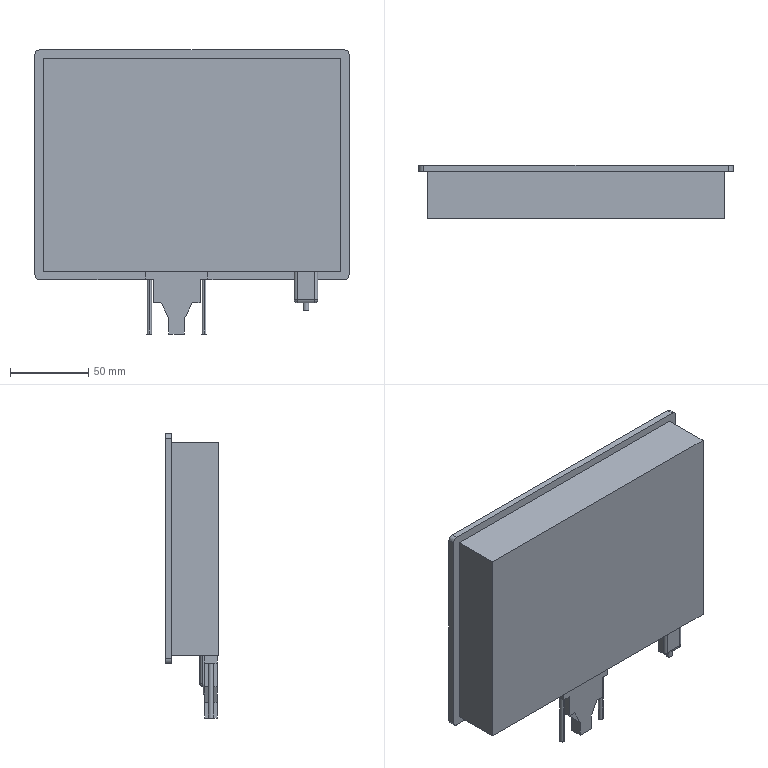Part | SolidWorks | features ICE 6, Cut 2, Fillet 2, Extrusion 1 | 1 solid | 69 faces | box 200.4 x 34 x 181.25 mm | volume 892134 mm3 | plane 47 | cylinder 18 | sphere 4 | commonest cylinder face diameters 4 x8 3 x4 6 x4 3.5 x2